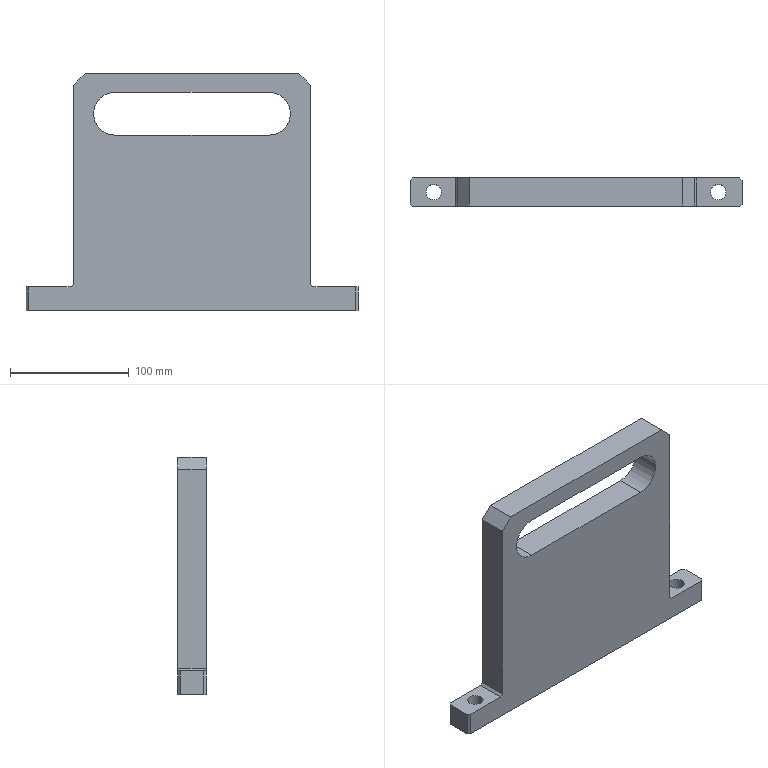Part | STEP file | 1 solid | 26 faces | box 280 x 24 x 200 mm | volume 853878 mm3 | plane 20 | cylinder 6 | commonest cylinder face diameters 13 x4 36 x2